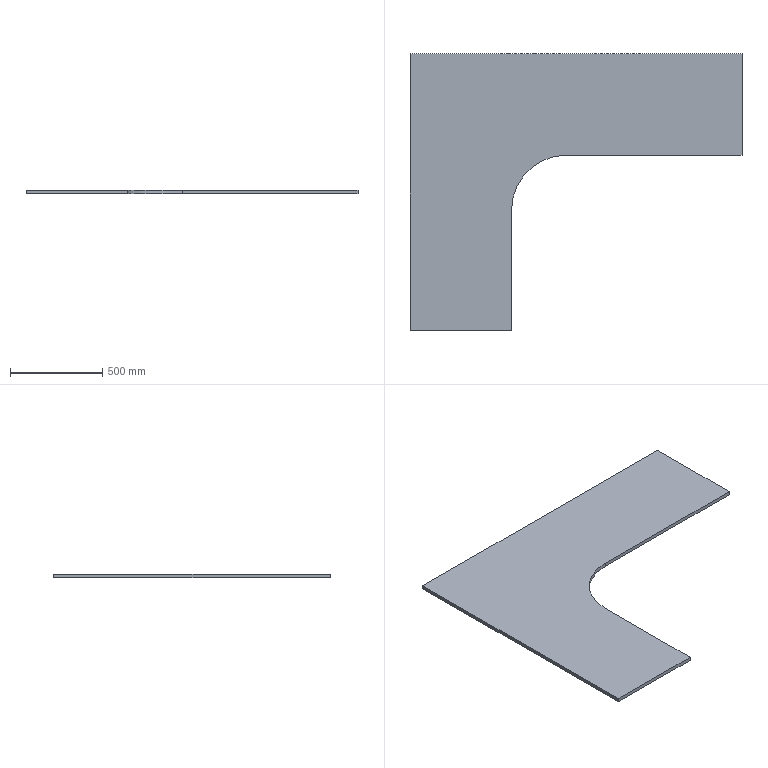Part | SolidWorks | features Extrusion 1 | 1 solid | 9 faces | box 1800 x 1500 x 20 mm | volume 30636283 mm3 | plane 8 | cylinder 1 | commonest cylinder face diameters 600 x1
STEP:
#1=CARTESIAN_POINT('',(0.,0.,0.));
#2=VERTEX_POINT('',#1);
#3=CARTESIAN_POINT('',(550.,0.,0.));
#4=VERTEX_POINT('',#3);
#5=CARTESIAN_POINT('',(550.,0.,0.));
#6=DIRECTION('',(1.,0.,0.));
#7=VECTOR('',#6,1000.);
#8=LINE('',#5,#7);
#9=EDGE_CURVE('',#2,#4,#8,.T.);
#10=ORIENTED_EDGE('',*,*,#9,.T.);
#11=CARTESIAN_POINT('',(550.,0.,20.));
#12=VERTEX_POINT('',#11);
#13=CARTESIAN_POINT('',(550.,0.,20.));
#14=DIRECTION('',(0.,0.,-1.));
#15=VECTOR('',#14,1000.);
#16=LINE('',#13,#15);
#17=EDGE_CURVE('',#12,#4,#16,.T.);
#18=ORIENTED_EDGE('',*,*,#17,.F.);
#19=CARTESIAN_POINT('',(0.,0.,20.));
#20=VERTEX_POINT('',#19);
#21=CARTESIAN_POINT('',(550.,0.,20.));
#22=DIRECTION('',(1.,0.,0.));
#23=VECTOR('',#22,1000.);
#24=LINE('',#21,#23);
#25=EDGE_CURVE('',#20,#12,#24,.T.);
#26=ORIENTED_EDGE('',*,*,#25,.F.);
#27=CARTESIAN_POINT('',(0.,0.,20.));
#28=DIRECTION('',(0.,0.,-1.));
#29=VECTOR('',#28,1000.);
#30=LINE('',#27,#29);
#31=EDGE_CURVE('',#20,#2,#30,.T.);
#32=ORIENTED_EDGE('',*,*,#31,.T.);
#33=EDGE_LOOP('',(#10,#18,#26,#32));
#34=FACE_OUTER_BOUND('',#33,.T.);
#35=CARTESIAN_POINT('',(550.,0.,20.));
#36=DIRECTION('',(0.,1.,0.));
#37=DIRECTION('',(-1.,0.,0.));
#38=AXIS2_PLACEMENT_3D('',#35,#36,#37);
#39=PLANE('',#38);
#40=ADVANCED_FACE('',(#34),#39,.F.);
#41=CARTESIAN_POINT('',(550.,650.,0.));
#42=VERTEX_POINT('',#41);
#43=CARTESIAN_POINT('',(550.,650.,0.));
#44=DIRECTION('',(0.,1.,0.));
#45=VECTOR('',#44,1000.);
#46=LINE('',#43,#45);
#47=EDGE_CURVE('',#4,#42,#46,.T.);
#48=ORIENTED_EDGE('',*,*,#47,.T.);
#49=CARTESIAN_POINT('',(550.,650.,20.));
#50=VERTEX_POINT('',#49);
#51=CARTESIAN_POINT('',(550.,650.,20.));
#52=DIRECTION('',(0.,0.,-1.));
#53=VECTOR('',#52,1000.);
#54=LINE('',#51,#53);
#55=EDGE_CURVE('',#50,#42,#54,.T.);
#56=ORIENTED_EDGE('',*,*,#55,.F.);
#57=CARTESIAN_POINT('',(550.,650.,20.));
#58=DIRECTION('',(0.,1.,0.));
#59=VECTOR('',#58,1000.);
#60=LINE('',#57,#59);
#61=EDGE_CURVE('',#12,#50,#60,.T.);
#62=ORIENTED_EDGE('',*,*,#61,.F.);
#63=ORIENTED_EDGE('',*,*,#17,.T.);
#64=EDGE_LOOP('',(#48,#56,#62,#63));
#65=FACE_OUTER_BOUND('',#64,.T.);
#66=CARTESIAN_POINT('',(550.,650.,20.));
#67=DIRECTION('',(-1.,0.,0.));
#68=DIRECTION('',(0.,0.,1.));
#69=AXIS2_PLACEMENT_3D('',#66,#67,#68);
#70=PLANE('',#69);
#71=ADVANCED_FACE('',(#65),#70,.F.);
#72=CARTESIAN_POINT('',(850.,950.,0.));
#73=VERTEX_POINT('',#72);
#74=CARTESIAN_POINT('',(850.,650.,0.));
#75=DIRECTION('',(0.,0.,-1.));
#76=DIRECTION('',(1.,0.,0.));
#77=AXIS2_PLACEMENT_3D('',#74,#75,#76);
#78=CIRCLE('',#77,300.);
#79=EDGE_CURVE('',#42,#73,#78,.T.);
#80=ORIENTED_EDGE('',*,*,#79,.T.);
#81=CARTESIAN_POINT('',(850.,950.,20.));
#82=VERTEX_POINT('',#81);
#83=CARTESIAN_POINT('',(850.,950.,20.));
#84=DIRECTION('',(0.,0.,-1.));
#85=VECTOR('',#84,1000.);
#86=LINE('',#83,#85);
#87=EDGE_CURVE('',#82,#73,#86,.T.);
#88=ORIENTED_EDGE('',*,*,#87,.F.);
#89=CARTESIAN_POINT('',(850.,650.,20.));
#90=DIRECTION('',(0.,0.,-1.));
#91=DIRECTION('',(1.,0.,0.));
#92=AXIS2_PLACEMENT_3D('',#89,#90,#91);
#93=CIRCLE('',#92,300.);
#94=EDGE_CURVE('',#50,#82,#93,.T.);
#95=ORIENTED_EDGE('',*,*,#94,.F.);
#96=ORIENTED_EDGE('',*,*,#55,.T.);
#97=EDGE_LOOP('',(#80,#88,#95,#96));
#98=FACE_OUTER_BOUND('',#97,.T.);
#99=CARTESIAN_POINT('',(850.,650.,20.));
#100=DIRECTION('',(0.,0.,-1.));
#101=DIRECTION('',(-1.,0.,0.));
#102=AXIS2_PLACEMENT_3D('',#99,#100,#101);
#103=CYLINDRICAL_SURFACE('',#102,300.);
#104=ADVANCED_FACE('',(#98),#103,.F.);
#105=CARTESIAN_POINT('',(1800.,950.,0.));
#106=VERTEX_POINT('',#105);
#107=CARTESIAN_POINT('',(1800.,950.,0.));
#108=DIRECTION('',(1.,0.,0.));
#109=VECTOR('',#108,1000.);
#110=LINE('',#107,#109);
#111=EDGE_CURVE('',#73,#106,#110,.T.);
#112=ORIENTED_EDGE('',*,*,#111,.T.);
#113=CARTESIAN_POINT('',(1800.,950.,20.));
#114=VERTEX_POINT('',#113);
#115=CARTESIAN_POINT('',(1800.,950.,20.));
#116=DIRECTION('',(0.,0.,-1.));
#117=VECTOR('',#116,1000.);
#118=LINE('',#115,#117);
#119=EDGE_CURVE('',#114,#106,#118,.T.);
#120=ORIENTED_EDGE('',*,*,#119,.F.);
#121=CARTESIAN_POINT('',(1800.,950.,20.));
#122=DIRECTION('',(1.,0.,0.));
#123=VECTOR('',#122,1000.);
#124=LINE('',#121,#123);
#125=EDGE_CURVE('',#82,#114,#124,.T.);
#126=ORIENTED_EDGE('',*,*,#125,.F.);
#127=ORIENTED_EDGE('',*,*,#87,.T.);
#128=EDGE_LOOP('',(#112,#120,#126,#127));
#129=FACE_OUTER_BOUND('',#128,.T.);
#130=CARTESIAN_POINT('',(1800.,950.,20.));
#131=DIRECTION('',(0.,1.,0.));
#132=DIRECTION('',(-1.,0.,0.));
#133=AXIS2_PLACEMENT_3D('',#130,#131,#132);
#134=PLANE('',#133);
#135=ADVANCED_FACE('',(#129),#134,.F.);
#136=CARTESIAN_POINT('',(1800.,1500.,0.));
#137=VERTEX_POINT('',#136);
#138=CARTESIAN_POINT('',(1800.,1500.,0.));
#139=DIRECTION('',(0.,1.,0.));
#140=VECTOR('',#139,1000.);
#141=LINE('',#138,#140);
#142=EDGE_CURVE('',#106,#137,#141,.T.);
#143=ORIENTED_EDGE('',*,*,#142,.T.);
#144=CARTESIAN_POINT('',(1800.,1500.,20.));
#145=VERTEX_POINT('',#144);
#146=CARTESIAN_POINT('',(1800.,1500.,20.));
#147=DIRECTION('',(0.,0.,-1.));
#148=VECTOR('',#147,1000.);
#149=LINE('',#146,#148);
#150=EDGE_CURVE('',#145,#137,#149,.T.);
#151=ORIENTED_EDGE('',*,*,#150,.F.);
#152=CARTESIAN_POINT('',(1800.,1500.,20.));
#153=DIRECTION('',(0.,1.,0.));
#154=VECTOR('',#153,1000.);
#155=LINE('',#152,#154);
#156=EDGE_CURVE('',#114,#145,#155,.T.);
#157=ORIENTED_EDGE('',*,*,#156,.F.);
#158=ORIENTED_EDGE('',*,*,#119,.T.);
#159=EDGE_LOOP('',(#143,#151,#157,#158));
#160=FACE_OUTER_BOUND('',#159,.T.);
#161=CARTESIAN_POINT('',(1800.,1500.,20.));
#162=DIRECTION('',(-1.,0.,0.));
#163=DIRECTION('',(0.,0.,1.));
#164=AXIS2_PLACEMENT_3D('',#161,#162,#163);
#165=PLANE('',#164);
#166=ADVANCED_FACE('',(#160),#165,.F.);
#167=CARTESIAN_POINT('',(0.,1500.,0.));
#168=VERTEX_POINT('',#167);
#169=CARTESIAN_POINT('',(0.,1500.,0.));
#170=DIRECTION('',(-1.,0.,0.));
#171=VECTOR('',#170,1000.);
#172=LINE('',#169,#171);
#173=EDGE_CURVE('',#137,#168,#172,.T.);
#174=ORIENTED_EDGE('',*,*,#173,.T.);
#175=CARTESIAN_POINT('',(0.,1500.,20.));
#176=VERTEX_POINT('',#175);
#177=CARTESIAN_POINT('',(0.,1500.,20.));
#178=DIRECTION('',(0.,0.,-1.));
#179=VECTOR('',#178,1000.);
#180=LINE('',#177,#179);
#181=EDGE_CURVE('',#176,#168,#180,.T.);
#182=ORIENTED_EDGE('',*,*,#181,.F.);
#183=CARTESIAN_POINT('',(0.,1500.,20.));
#184=DIRECTION('',(-1.,0.,0.));
#185=VECTOR('',#184,1000.);
#186=LINE('',#183,#185);
#187=EDGE_CURVE('',#145,#176,#186,.T.);
#188=ORIENTED_EDGE('',*,*,#187,.F.);
#189=ORIENTED_EDGE('',*,*,#150,.T.);
#190=EDGE_LOOP('',(#174,#182,#188,#189));
#191=FACE_OUTER_BOUND('',#190,.T.);
#192=CARTESIAN_POINT('',(0.,1500.,20.));
#193=DIRECTION('',(0.,-1.,0.));
#194=DIRECTION('',(0.,0.,-1.));
#195=AXIS2_PLACEMENT_3D('',#192,#193,#194);
#196=PLANE('',#195);
#197=ADVANCED_FACE('',(#191),#196,.F.);
#198=CARTESIAN_POINT('',(0.,0.,0.));
#199=DIRECTION('',(0.,-1.,0.));
#200=VECTOR('',#199,1000.);
#201=LINE('',#198,#200);
#202=EDGE_CURVE('',#168,#2,#201,.T.);
#203=ORIENTED_EDGE('',*,*,#202,.T.);
#204=ORIENTED_EDGE('',*,*,#31,.F.);
#205=CARTESIAN_POINT('',(0.,0.,20.));
#206=DIRECTION('',(0.,-1.,0.));
#207=VECTOR('',#206,1000.);
#208=LINE('',#205,#207);
#209=EDGE_CURVE('',#176,#20,#208,.T.);
#210=ORIENTED_EDGE('',*,*,#209,.F.);
#211=ORIENTED_EDGE('',*,*,#181,.T.);
#212=EDGE_LOOP('',(#203,#204,#210,#211));
#213=FACE_OUTER_BOUND('',#212,.T.);
#214=CARTESIAN_POINT('',(0.,0.,20.));
#215=DIRECTION('',(1.,0.,0.));
#216=DIRECTION('',(0.,0.,-1.));
#217=AXIS2_PLACEMENT_3D('',#214,#215,#216);
#218=PLANE('',#217);
#219=ADVANCED_FACE('',(#213),#218,.F.);
#220=ORIENTED_EDGE('',*,*,#25,.T.);
#221=ORIENTED_EDGE('',*,*,#61,.T.);
#222=ORIENTED_EDGE('',*,*,#94,.T.);
#223=ORIENTED_EDGE('',*,*,#125,.T.);
#224=ORIENTED_EDGE('',*,*,#156,.T.);
#225=ORIENTED_EDGE('',*,*,#187,.T.);
#226=ORIENTED_EDGE('',*,*,#209,.T.);
#227=EDGE_LOOP('',(#220,#221,#222,#223,#224,#225,#226));
#228=FACE_OUTER_BOUND('',#227,.T.);
#229=CARTESIAN_POINT('',(850.,650.,20.));
#230=DIRECTION('',(0.,0.,1.));
#231=DIRECTION('',(1.,0.,0.));
#232=AXIS2_PLACEMENT_3D('',#229,#230,#231);
#233=PLANE('',#232);
#234=ADVANCED_FACE('',(#228),#233,.T.);
#235=ORIENTED_EDGE('',*,*,#9,.F.);
#236=ORIENTED_EDGE('',*,*,#202,.F.);
#237=ORIENTED_EDGE('',*,*,#173,.F.);
#238=ORIENTED_EDGE('',*,*,#142,.F.);
#239=ORIENTED_EDGE('',*,*,#111,.F.);
#240=ORIENTED_EDGE('',*,*,#79,.F.);
#241=ORIENTED_EDGE('',*,*,#47,.F.);
#242=EDGE_LOOP('',(#235,#236,#237,#238,#239,#240,#241));
#243=FACE_OUTER_BOUND('',#242,.T.);
#244=CARTESIAN_POINT('',(850.,650.,0.));
#245=DIRECTION('',(0.,0.,1.));
#246=DIRECTION('',(1.,0.,0.));
#247=AXIS2_PLACEMENT_3D('',#244,#245,#246);
#248=PLANE('',#247);
#249=ADVANCED_FACE('',(#243),#248,.F.);
#250=CLOSED_SHELL('',(#40,#71,#104,#135,#166,#197,#219,#234,#249));
#251=MANIFOLD_SOLID_BREP('',#250);
#252=CARTESIAN_POINT('',(0.,0.,0.));
#253=DIRECTION('',(0.,0.,1.));
#254=DIRECTION('',(1.,0.,0.));
#255=AXIS2_PLACEMENT_3D('',#252,#253,#254);
#256=(LENGTH_UNIT()NAMED_UNIT(*)SI_UNIT(.MILLI.,.METRE.));
#257=UNCERTAINTY_MEASURE_WITH_UNIT(LENGTH_MEASURE(0.00001),#256,'','');
#258=(NAMED_UNIT(*)PLANE_ANGLE_UNIT()SI_UNIT($,.RADIAN.));
#259=(NAMED_UNIT(*)SI_UNIT($,.STERADIAN.)SOLID_ANGLE_UNIT());
#260=(GEOMETRIC_REPRESENTATION_CONTEXT(3)GLOBAL_UNCERTAINTY_ASSIGNED_CONTEXT((#257))GLOBAL_UNIT_ASSIGNED_CONTEXT((#256,#258,#259))REPRESENTATION_CONTEXT('',''));
#261=ADVANCED_BREP_SHAPE_REPRESENTATION('',(#251,#255),#260);